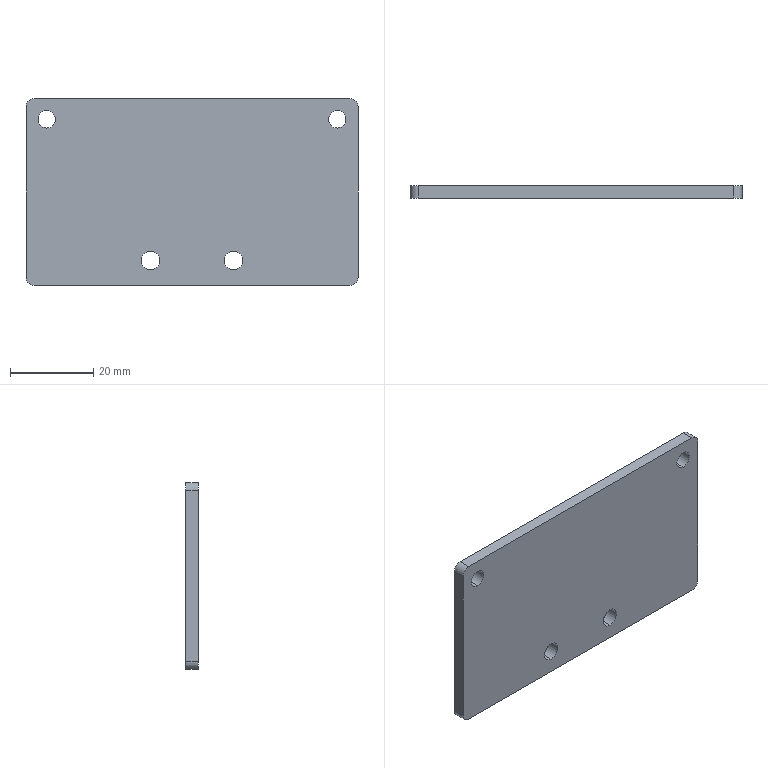Part | STEP file | ND25021-01-JDKM-07-BJ | 1 solid | 18 faces | box 80 x 3 x 45 mm | volume 10611 mm3 | cylinder 12 | plane 6 | commonest cylinder face diameters 4 x4 4.2 x4 4.5 x4